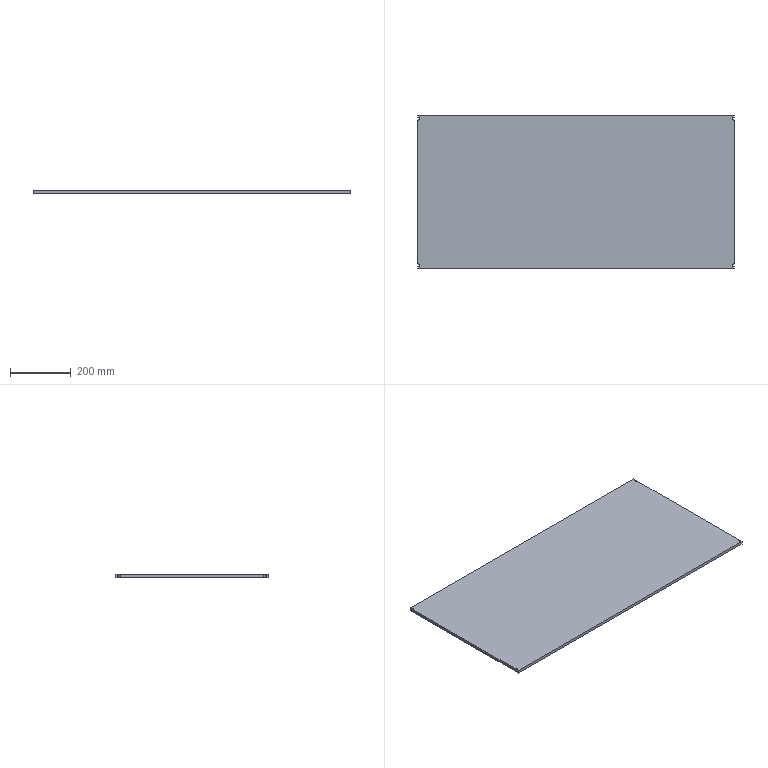Part | STEP file | 750038236 | 1 solid | 16 faces | box 1044 x 507 x 10 mm | volume 5291709 mm3 | plane 10 | cylinder 6 | commonest cylinder face diameters 10 x6
STEP:
#1=CARTESIAN_POINT('',(-517.5,-242.5,0.));
#2=VERTEX_POINT('',#1);
#3=CARTESIAN_POINT('',(-522.,-237.525,0.));
#4=VERTEX_POINT('',#3);
#5=CARTESIAN_POINT('',(-522.5,-242.5,0.));
#6=DIRECTION('',(0.,0.,1.));
#7=DIRECTION('',(1.,0.,0.));
#8=AXIS2_PLACEMENT_3D('',#5,#6,#7);
#9=CIRCLE('',#8,5.);
#10=EDGE_CURVE('',#2,#4,#9,.T.);
#11=ORIENTED_EDGE('',*,*,#10,.F.);
#12=CARTESIAN_POINT('',(-517.5,-242.5,10.));
#13=VERTEX_POINT('',#12);
#14=CARTESIAN_POINT('',(-517.5,-242.5,-54990.));
#15=DIRECTION('',(0.,0.,1.));
#16=VECTOR('',#15,1000.);
#17=LINE('',#14,#16);
#18=EDGE_CURVE('',#2,#13,#17,.T.);
#19=ORIENTED_EDGE('',*,*,#18,.T.);
#20=CARTESIAN_POINT('',(-522.,-237.525,10.));
#21=VERTEX_POINT('',#20);
#22=CARTESIAN_POINT('',(-522.5,-242.5,10.));
#23=DIRECTION('',(0.,0.,-1.));
#24=DIRECTION('',(1.,0.,0.));
#25=AXIS2_PLACEMENT_3D('',#22,#23,#24);
#26=CIRCLE('',#25,5.);
#27=EDGE_CURVE('',#21,#13,#26,.T.);
#28=ORIENTED_EDGE('',*,*,#27,.F.);
#29=CARTESIAN_POINT('',(-522.,-237.525,-54990.));
#30=DIRECTION('',(0.,0.,1.));
#31=VECTOR('',#30,1000.);
#32=LINE('',#29,#31);
#33=EDGE_CURVE('',#4,#21,#32,.T.);
#34=ORIENTED_EDGE('',*,*,#33,.F.);
#35=EDGE_LOOP('',(#11,#19,#28,#34));
#36=FACE_OUTER_BOUND('',#35,.T.);
#37=CARTESIAN_POINT('',(-522.5,-242.5,-54990.));
#38=DIRECTION('',(0.,0.,1.));
#39=DIRECTION('',(1.,0.,0.));
#40=AXIS2_PLACEMENT_3D('',#37,#38,#39);
#41=CYLINDRICAL_SURFACE('',#40,5.);
#42=ADVANCED_FACE('',(#36),#41,.F.);
#43=CARTESIAN_POINT('',(-517.5,242.5,0.));
#44=VERTEX_POINT('',#43);
#45=CARTESIAN_POINT('',(-522.,247.475,0.));
#46=VERTEX_POINT('',#45);
#47=CARTESIAN_POINT('',(-522.5,242.5,0.));
#48=DIRECTION('',(0.,0.,1.));
#49=DIRECTION('',(1.,0.,0.));
#50=AXIS2_PLACEMENT_3D('',#47,#48,#49);
#51=CIRCLE('',#50,5.);
#52=EDGE_CURVE('',#44,#46,#51,.T.);
#53=ORIENTED_EDGE('',*,*,#52,.F.);
#54=CARTESIAN_POINT('',(-517.5,242.5,10.));
#55=VERTEX_POINT('',#54);
#56=CARTESIAN_POINT('',(-517.5,242.5,-54990.));
#57=DIRECTION('',(0.,0.,1.));
#58=VECTOR('',#57,1000.);
#59=LINE('',#56,#58);
#60=EDGE_CURVE('',#44,#55,#59,.T.);
#61=ORIENTED_EDGE('',*,*,#60,.T.);
#62=CARTESIAN_POINT('',(-522.,247.475,10.));
#63=VERTEX_POINT('',#62);
#64=CARTESIAN_POINT('',(-522.5,242.5,10.));
#65=DIRECTION('',(0.,0.,-1.));
#66=DIRECTION('',(1.,0.,0.));
#67=AXIS2_PLACEMENT_3D('',#64,#65,#66);
#68=CIRCLE('',#67,5.);
#69=EDGE_CURVE('',#63,#55,#68,.T.);
#70=ORIENTED_EDGE('',*,*,#69,.F.);
#71=CARTESIAN_POINT('',(-522.,247.475,-54990.));
#72=DIRECTION('',(0.,0.,1.));
#73=VECTOR('',#72,1000.);
#74=LINE('',#71,#73);
#75=EDGE_CURVE('',#46,#63,#74,.T.);
#76=ORIENTED_EDGE('',*,*,#75,.F.);
#77=EDGE_LOOP('',(#53,#61,#70,#76));
#78=FACE_OUTER_BOUND('',#77,.T.);
#79=CARTESIAN_POINT('',(-522.5,242.5,-54990.));
#80=DIRECTION('',(0.,0.,1.));
#81=DIRECTION('',(1.,0.,0.));
#82=AXIS2_PLACEMENT_3D('',#79,#80,#81);
#83=CYLINDRICAL_SURFACE('',#82,5.);
#84=ADVANCED_FACE('',(#78),#83,.F.);
#85=CARTESIAN_POINT('',(-522.,-253.5,10.));
#86=VERTEX_POINT('',#85);
#87=CARTESIAN_POINT('',(522.,-253.5,10.));
#88=VERTEX_POINT('',#87);
#89=CARTESIAN_POINT('',(0.,-253.5,10.));
#90=DIRECTION('',(1.,0.,0.));
#91=VECTOR('',#90,1000.);
#92=LINE('',#89,#91);
#93=EDGE_CURVE('',#86,#88,#92,.T.);
#94=ORIENTED_EDGE('',*,*,#93,.T.);
#95=CARTESIAN_POINT('',(522.,-247.475,10.));
#96=VERTEX_POINT('',#95);
#97=CARTESIAN_POINT('',(522.,0.,10.));
#98=DIRECTION('',(0.,1.,0.));
#99=VECTOR('',#98,1000.);
#100=LINE('',#97,#99);
#101=EDGE_CURVE('',#88,#96,#100,.T.);
#102=ORIENTED_EDGE('',*,*,#101,.T.);
#103=CARTESIAN_POINT('',(522.,-237.525,10.));
#104=VERTEX_POINT('',#103);
#105=CARTESIAN_POINT('',(522.5,-242.5,10.));
#106=DIRECTION('',(0.,0.,-1.));
#107=DIRECTION('',(1.,0.,0.));
#108=AXIS2_PLACEMENT_3D('',#105,#106,#107);
#109=CIRCLE('',#108,5.);
#110=EDGE_CURVE('',#96,#104,#109,.T.);
#111=ORIENTED_EDGE('',*,*,#110,.T.);
#112=CARTESIAN_POINT('',(522.,237.525,10.));
#113=VERTEX_POINT('',#112);
#114=CARTESIAN_POINT('',(522.,0.,10.));
#115=DIRECTION('',(0.,1.,0.));
#116=VECTOR('',#115,1000.);
#117=LINE('',#114,#116);
#118=EDGE_CURVE('',#104,#113,#117,.T.);
#119=ORIENTED_EDGE('',*,*,#118,.T.);
#120=CARTESIAN_POINT('',(522.,247.475,10.));
#121=VERTEX_POINT('',#120);
#122=CARTESIAN_POINT('',(522.5,242.5,10.));
#123=DIRECTION('',(0.,0.,-1.));
#124=DIRECTION('',(1.,0.,0.));
#125=AXIS2_PLACEMENT_3D('',#122,#123,#124);
#126=CIRCLE('',#125,5.);
#127=EDGE_CURVE('',#113,#121,#126,.T.);
#128=ORIENTED_EDGE('',*,*,#127,.T.);
#129=CARTESIAN_POINT('',(522.,253.5,10.));
#130=VERTEX_POINT('',#129);
#131=CARTESIAN_POINT('',(522.,0.,10.));
#132=DIRECTION('',(0.,1.,0.));
#133=VECTOR('',#132,1000.);
#134=LINE('',#131,#133);
#135=EDGE_CURVE('',#121,#130,#134,.T.);
#136=ORIENTED_EDGE('',*,*,#135,.T.);
#137=CARTESIAN_POINT('',(-522.,253.5,10.));
#138=VERTEX_POINT('',#137);
#139=CARTESIAN_POINT('',(0.,253.5,10.));
#140=DIRECTION('',(-1.,0.,0.));
#141=VECTOR('',#140,1000.);
#142=LINE('',#139,#141);
#143=EDGE_CURVE('',#130,#138,#142,.T.);
#144=ORIENTED_EDGE('',*,*,#143,.T.);
#145=CARTESIAN_POINT('',(-522.,0.,10.));
#146=DIRECTION('',(0.,-1.,0.));
#147=VECTOR('',#146,1000.);
#148=LINE('',#145,#147);
#149=EDGE_CURVE('',#138,#63,#148,.T.);
#150=ORIENTED_EDGE('',*,*,#149,.T.);
#151=ORIENTED_EDGE('',*,*,#69,.T.);
#152=CARTESIAN_POINT('',(-522.,237.525,10.));
#153=VERTEX_POINT('',#152);
#154=CARTESIAN_POINT('',(-522.5,242.5,10.));
#155=DIRECTION('',(0.,0.,-1.));
#156=DIRECTION('',(1.,0.,0.));
#157=AXIS2_PLACEMENT_3D('',#154,#155,#156);
#158=CIRCLE('',#157,5.);
#159=EDGE_CURVE('',#55,#153,#158,.T.);
#160=ORIENTED_EDGE('',*,*,#159,.T.);
#161=CARTESIAN_POINT('',(-522.,0.,10.));
#162=DIRECTION('',(0.,-1.,0.));
#163=VECTOR('',#162,1000.);
#164=LINE('',#161,#163);
#165=EDGE_CURVE('',#153,#21,#164,.T.);
#166=ORIENTED_EDGE('',*,*,#165,.T.);
#167=ORIENTED_EDGE('',*,*,#27,.T.);
#168=CARTESIAN_POINT('',(-522.,-247.475,10.));
#169=VERTEX_POINT('',#168);
#170=CARTESIAN_POINT('',(-522.5,-242.5,10.));
#171=DIRECTION('',(0.,0.,-1.));
#172=DIRECTION('',(1.,0.,0.));
#173=AXIS2_PLACEMENT_3D('',#170,#171,#172);
#174=CIRCLE('',#173,5.);
#175=EDGE_CURVE('',#13,#169,#174,.T.);
#176=ORIENTED_EDGE('',*,*,#175,.T.);
#177=CARTESIAN_POINT('',(-522.,0.,10.));
#178=DIRECTION('',(0.,-1.,0.));
#179=VECTOR('',#178,1000.);
#180=LINE('',#177,#179);
#181=EDGE_CURVE('',#169,#86,#180,.T.);
#182=ORIENTED_EDGE('',*,*,#181,.T.);
#183=EDGE_LOOP('',(#94,#102,#111,#119,#128,#136,#144,#150,#151,#160,#166,#167,#176,#182));
#184=FACE_OUTER_BOUND('',#183,.T.);
#185=CARTESIAN_POINT('',(0.,0.,10.));
#186=DIRECTION('',(0.,0.,1.));
#187=DIRECTION('',(1.,0.,0.));
#188=AXIS2_PLACEMENT_3D('',#185,#186,#187);
#189=PLANE('',#188);
#190=ADVANCED_FACE('',(#184),#189,.T.);
#191=CARTESIAN_POINT('',(522.,-247.475,0.));
#192=VERTEX_POINT('',#191);
#193=CARTESIAN_POINT('',(522.,-247.475,10.));
#194=DIRECTION('',(0.,0.,-1.));
#195=VECTOR('',#194,1000.);
#196=LINE('',#193,#195);
#197=EDGE_CURVE('',#96,#192,#196,.T.);
#198=ORIENTED_EDGE('',*,*,#197,.F.);
#199=ORIENTED_EDGE('',*,*,#101,.F.);
#200=CARTESIAN_POINT('',(522.,-253.5,0.));
#201=VERTEX_POINT('',#200);
#202=CARTESIAN_POINT('',(522.,-253.5,10.));
#203=DIRECTION('',(0.,0.,1.));
#204=VECTOR('',#203,1000.);
#205=LINE('',#202,#204);
#206=EDGE_CURVE('',#201,#88,#205,.T.);
#207=ORIENTED_EDGE('',*,*,#206,.F.);
#208=CARTESIAN_POINT('',(522.,-253.5,0.));
#209=DIRECTION('',(0.,-1.,0.));
#210=VECTOR('',#209,1000.);
#211=LINE('',#208,#210);
#212=EDGE_CURVE('',#192,#201,#211,.T.);
#213=ORIENTED_EDGE('',*,*,#212,.F.);
#214=EDGE_LOOP('',(#198,#199,#207,#213));
#215=FACE_OUTER_BOUND('',#214,.T.);
#216=CARTESIAN_POINT('',(522.,-253.5,10.));
#217=DIRECTION('',(-1.,0.,0.));
#218=DIRECTION('',(0.,0.,1.));
#219=AXIS2_PLACEMENT_3D('',#216,#217,#218);
#220=PLANE('',#219);
#221=ADVANCED_FACE('',(#215),#220,.F.);
#222=ORIENTED_EDGE('',*,*,#206,.T.);
#223=ORIENTED_EDGE('',*,*,#93,.F.);
#224=CARTESIAN_POINT('',(-522.,-253.5,0.));
#225=VERTEX_POINT('',#224);
#226=CARTESIAN_POINT('',(-522.,-253.5,10.));
#227=DIRECTION('',(0.,0.,1.));
#228=VECTOR('',#227,1000.);
#229=LINE('',#226,#228);
#230=EDGE_CURVE('',#225,#86,#229,.T.);
#231=ORIENTED_EDGE('',*,*,#230,.F.);
#232=CARTESIAN_POINT('',(-522.,-253.5,0.));
#233=DIRECTION('',(-1.,0.,0.));
#234=VECTOR('',#233,1000.);
#235=LINE('',#232,#234);
#236=EDGE_CURVE('',#201,#225,#235,.T.);
#237=ORIENTED_EDGE('',*,*,#236,.F.);
#238=EDGE_LOOP('',(#222,#223,#231,#237));
#239=FACE_OUTER_BOUND('',#238,.T.);
#240=CARTESIAN_POINT('',(-522.,-253.5,10.));
#241=DIRECTION('',(0.,1.,0.));
#242=DIRECTION('',(0.,0.,1.));
#243=AXIS2_PLACEMENT_3D('',#240,#241,#242);
#244=PLANE('',#243);
#245=ADVANCED_FACE('',(#239),#244,.F.);
#246=CARTESIAN_POINT('',(-522.,-247.475,0.));
#247=VERTEX_POINT('',#246);
#248=CARTESIAN_POINT('',(-522.,-247.475,10.));
#249=DIRECTION('',(0.,0.,1.));
#250=VECTOR('',#249,1000.);
#251=LINE('',#248,#250);
#252=EDGE_CURVE('',#247,#169,#251,.T.);
#253=ORIENTED_EDGE('',*,*,#252,.F.);
#254=CARTESIAN_POINT('',(-522.,253.5,0.));
#255=DIRECTION('',(0.,1.,0.));
#256=VECTOR('',#255,1000.);
#257=LINE('',#254,#256);
#258=EDGE_CURVE('',#225,#247,#257,.T.);
#259=ORIENTED_EDGE('',*,*,#258,.F.);
#260=ORIENTED_EDGE('',*,*,#230,.T.);
#261=ORIENTED_EDGE('',*,*,#181,.F.);
#262=EDGE_LOOP('',(#253,#259,#260,#261));
#263=FACE_OUTER_BOUND('',#262,.T.);
#264=CARTESIAN_POINT('',(-522.,253.5,10.));
#265=DIRECTION('',(1.,0.,0.));
#266=DIRECTION('',(0.,0.,-1.));
#267=AXIS2_PLACEMENT_3D('',#264,#265,#266);
#268=PLANE('',#267);
#269=ADVANCED_FACE('',(#263),#268,.F.);
#270=ORIENTED_EDGE('',*,*,#18,.F.);
#271=CARTESIAN_POINT('',(-522.5,-242.5,0.));
#272=DIRECTION('',(0.,0.,1.));
#273=DIRECTION('',(1.,0.,0.));
#274=AXIS2_PLACEMENT_3D('',#271,#272,#273);
#275=CIRCLE('',#274,5.);
#276=EDGE_CURVE('',#247,#2,#275,.T.);
#277=ORIENTED_EDGE('',*,*,#276,.F.);
#278=ORIENTED_EDGE('',*,*,#252,.T.);
#279=ORIENTED_EDGE('',*,*,#175,.F.);
#280=EDGE_LOOP('',(#270,#277,#278,#279));
#281=FACE_OUTER_BOUND('',#280,.T.);
#282=CARTESIAN_POINT('',(-522.5,-242.5,-54990.));
#283=DIRECTION('',(0.,0.,1.));
#284=DIRECTION('',(1.,0.,0.));
#285=AXIS2_PLACEMENT_3D('',#282,#283,#284);
#286=CYLINDRICAL_SURFACE('',#285,5.);
#287=ADVANCED_FACE('',(#281),#286,.F.);
#288=CARTESIAN_POINT('',(-522.,237.525,0.));
#289=VERTEX_POINT('',#288);
#290=CARTESIAN_POINT('',(-522.,237.525,10.));
#291=DIRECTION('',(0.,0.,1.));
#292=VECTOR('',#291,1000.);
#293=LINE('',#290,#292);
#294=EDGE_CURVE('',#289,#153,#293,.T.);
#295=ORIENTED_EDGE('',*,*,#294,.F.);
#296=CARTESIAN_POINT('',(-522.,253.5,0.));
#297=DIRECTION('',(0.,1.,0.));
#298=VECTOR('',#297,1000.);
#299=LINE('',#296,#298);
#300=EDGE_CURVE('',#4,#289,#299,.T.);
#301=ORIENTED_EDGE('',*,*,#300,.F.);
#302=ORIENTED_EDGE('',*,*,#33,.T.);
#303=ORIENTED_EDGE('',*,*,#165,.F.);
#304=EDGE_LOOP('',(#295,#301,#302,#303));
#305=FACE_OUTER_BOUND('',#304,.T.);
#306=CARTESIAN_POINT('',(-522.,253.5,10.));
#307=DIRECTION('',(1.,0.,0.));
#308=DIRECTION('',(0.,0.,-1.));
#309=AXIS2_PLACEMENT_3D('',#306,#307,#308);
#310=PLANE('',#309);
#311=ADVANCED_FACE('',(#305),#310,.F.);
#312=ORIENTED_EDGE('',*,*,#60,.F.);
#313=CARTESIAN_POINT('',(-522.5,242.5,0.));
#314=DIRECTION('',(0.,0.,1.));
#315=DIRECTION('',(1.,0.,0.));
#316=AXIS2_PLACEMENT_3D('',#313,#314,#315);
#317=CIRCLE('',#316,5.);
#318=EDGE_CURVE('',#289,#44,#317,.T.);
#319=ORIENTED_EDGE('',*,*,#318,.F.);
#320=ORIENTED_EDGE('',*,*,#294,.T.);
#321=ORIENTED_EDGE('',*,*,#159,.F.);
#322=EDGE_LOOP('',(#312,#319,#320,#321));
#323=FACE_OUTER_BOUND('',#322,.T.);
#324=CARTESIAN_POINT('',(-522.5,242.5,-54990.));
#325=DIRECTION('',(0.,0.,1.));
#326=DIRECTION('',(1.,0.,0.));
#327=AXIS2_PLACEMENT_3D('',#324,#325,#326);
#328=CYLINDRICAL_SURFACE('',#327,5.);
#329=ADVANCED_FACE('',(#323),#328,.F.);
#330=ORIENTED_EDGE('',*,*,#75,.T.);
#331=ORIENTED_EDGE('',*,*,#149,.F.);
#332=CARTESIAN_POINT('',(-522.,253.5,0.));
#333=VERTEX_POINT('',#332);
#334=CARTESIAN_POINT('',(-522.,253.5,10.));
#335=DIRECTION('',(0.,0.,1.));
#336=VECTOR('',#335,1000.);
#337=LINE('',#334,#336);
#338=EDGE_CURVE('',#333,#138,#337,.T.);
#339=ORIENTED_EDGE('',*,*,#338,.F.);
#340=CARTESIAN_POINT('',(-522.,253.5,0.));
#341=DIRECTION('',(0.,1.,0.));
#342=VECTOR('',#341,1000.);
#343=LINE('',#340,#342);
#344=EDGE_CURVE('',#46,#333,#343,.T.);
#345=ORIENTED_EDGE('',*,*,#344,.F.);
#346=EDGE_LOOP('',(#330,#331,#339,#345));
#347=FACE_OUTER_BOUND('',#346,.T.);
#348=CARTESIAN_POINT('',(-522.,253.5,10.));
#349=DIRECTION('',(1.,0.,0.));
#350=DIRECTION('',(0.,0.,-1.));
#351=AXIS2_PLACEMENT_3D('',#348,#349,#350);
#352=PLANE('',#351);
#353=ADVANCED_FACE('',(#347),#352,.F.);
#354=ORIENTED_EDGE('',*,*,#338,.T.);
#355=ORIENTED_EDGE('',*,*,#143,.F.);
#356=CARTESIAN_POINT('',(522.,253.5,0.));
#357=VERTEX_POINT('',#356);
#358=CARTESIAN_POINT('',(522.,253.5,10.));
#359=DIRECTION('',(0.,0.,1.));
#360=VECTOR('',#359,1000.);
#361=LINE('',#358,#360);
#362=EDGE_CURVE('',#357,#130,#361,.T.);
#363=ORIENTED_EDGE('',*,*,#362,.F.);
#364=CARTESIAN_POINT('',(522.,253.5,0.));
#365=DIRECTION('',(1.,0.,0.));
#366=VECTOR('',#365,1000.);
#367=LINE('',#364,#366);
#368=EDGE_CURVE('',#333,#357,#367,.T.);
#369=ORIENTED_EDGE('',*,*,#368,.F.);
#370=EDGE_LOOP('',(#354,#355,#363,#369));
#371=FACE_OUTER_BOUND('',#370,.T.);
#372=CARTESIAN_POINT('',(522.,253.5,10.));
#373=DIRECTION('',(0.,-1.,0.));
#374=DIRECTION('',(0.,0.,-1.));
#375=AXIS2_PLACEMENT_3D('',#372,#373,#374);
#376=PLANE('',#375);
#377=ADVANCED_FACE('',(#371),#376,.F.);
#378=CARTESIAN_POINT('',(522.,247.475,0.));
#379=VERTEX_POINT('',#378);
#380=CARTESIAN_POINT('',(522.,247.475,10.));
#381=DIRECTION('',(0.,0.,1.));
#382=VECTOR('',#381,1000.);
#383=LINE('',#380,#382);
#384=EDGE_CURVE('',#379,#121,#383,.T.);
#385=ORIENTED_EDGE('',*,*,#384,.F.);
#386=CARTESIAN_POINT('',(522.,-253.5,0.));
#387=DIRECTION('',(0.,-1.,0.));
#388=VECTOR('',#387,1000.);
#389=LINE('',#386,#388);
#390=EDGE_CURVE('',#357,#379,#389,.T.);
#391=ORIENTED_EDGE('',*,*,#390,.F.);
#392=ORIENTED_EDGE('',*,*,#362,.T.);
#393=ORIENTED_EDGE('',*,*,#135,.F.);
#394=EDGE_LOOP('',(#385,#391,#392,#393));
#395=FACE_OUTER_BOUND('',#394,.T.);
#396=CARTESIAN_POINT('',(522.,-253.5,10.));
#397=DIRECTION('',(-1.,0.,0.));
#398=DIRECTION('',(0.,0.,1.));
#399=AXIS2_PLACEMENT_3D('',#396,#397,#398);
#400=PLANE('',#399);
#401=ADVANCED_FACE('',(#395),#400,.F.);
#402=ORIENTED_EDGE('',*,*,#384,.T.);
#403=ORIENTED_EDGE('',*,*,#127,.F.);
#404=CARTESIAN_POINT('',(522.,237.525,0.));
#405=VERTEX_POINT('',#404);
#406=CARTESIAN_POINT('',(522.,237.525,-54990.));
#407=DIRECTION('',(0.,0.,1.));
#408=VECTOR('',#407,1000.);
#409=LINE('',#406,#408);
#410=EDGE_CURVE('',#405,#113,#409,.T.);
#411=ORIENTED_EDGE('',*,*,#410,.F.);
#412=CARTESIAN_POINT('',(522.5,242.5,0.));
#413=DIRECTION('',(0.,0.,1.));
#414=DIRECTION('',(1.,0.,0.));
#415=AXIS2_PLACEMENT_3D('',#412,#413,#414);
#416=CIRCLE('',#415,5.);
#417=EDGE_CURVE('',#379,#405,#416,.T.);
#418=ORIENTED_EDGE('',*,*,#417,.F.);
#419=EDGE_LOOP('',(#402,#403,#411,#418));
#420=FACE_OUTER_BOUND('',#419,.T.);
#421=CARTESIAN_POINT('',(522.5,242.5,-54990.));
#422=DIRECTION('',(0.,0.,1.));
#423=DIRECTION('',(1.,0.,0.));
#424=AXIS2_PLACEMENT_3D('',#421,#422,#423);
#425=CYLINDRICAL_SURFACE('',#424,5.);
#426=ADVANCED_FACE('',(#420),#425,.F.);
#427=CARTESIAN_POINT('',(522.,-237.525,0.));
#428=VERTEX_POINT('',#427);
#429=CARTESIAN_POINT('',(522.,-237.525,10.));
#430=DIRECTION('',(0.,0.,1.));
#431=VECTOR('',#430,1000.);
#432=LINE('',#429,#431);
#433=EDGE_CURVE('',#428,#104,#432,.T.);
#434=ORIENTED_EDGE('',*,*,#433,.F.);
#435=CARTESIAN_POINT('',(522.,-253.5,0.));
#436=DIRECTION('',(0.,-1.,0.));
#437=VECTOR('',#436,1000.);
#438=LINE('',#435,#437);
#439=EDGE_CURVE('',#405,#428,#438,.T.);
#440=ORIENTED_EDGE('',*,*,#439,.F.);
#441=ORIENTED_EDGE('',*,*,#410,.T.);
#442=ORIENTED_EDGE('',*,*,#118,.F.);
#443=EDGE_LOOP('',(#434,#440,#441,#442));
#444=FACE_OUTER_BOUND('',#443,.T.);
#445=CARTESIAN_POINT('',(522.,-253.5,10.));
#446=DIRECTION('',(-1.,0.,0.));
#447=DIRECTION('',(0.,0.,1.));
#448=AXIS2_PLACEMENT_3D('',#445,#446,#447);
#449=PLANE('',#448);
#450=ADVANCED_FACE('',(#444),#449,.F.);
#451=ORIENTED_EDGE('',*,*,#433,.T.);
#452=ORIENTED_EDGE('',*,*,#110,.F.);
#453=ORIENTED_EDGE('',*,*,#197,.T.);
#454=CARTESIAN_POINT('',(522.5,-242.5,0.));
#455=DIRECTION('',(0.,0.,1.));
#456=DIRECTION('',(1.,0.,0.));
#457=AXIS2_PLACEMENT_3D('',#454,#455,#456);
#458=CIRCLE('',#457,5.);
#459=EDGE_CURVE('',#428,#192,#458,.T.);
#460=ORIENTED_EDGE('',*,*,#459,.F.);
#461=EDGE_LOOP('',(#451,#452,#453,#460));
#462=FACE_OUTER_BOUND('',#461,.T.);
#463=CARTESIAN_POINT('',(522.5,-242.5,-54990.));
#464=DIRECTION('',(0.,0.,1.));
#465=DIRECTION('',(1.,0.,0.));
#466=AXIS2_PLACEMENT_3D('',#463,#464,#465);
#467=CYLINDRICAL_SURFACE('',#466,5.);
#468=ADVANCED_FACE('',(#462),#467,.F.);
#469=ORIENTED_EDGE('',*,*,#459,.T.);
#470=ORIENTED_EDGE('',*,*,#212,.T.);
#471=ORIENTED_EDGE('',*,*,#236,.T.);
#472=ORIENTED_EDGE('',*,*,#258,.T.);
#473=ORIENTED_EDGE('',*,*,#276,.T.);
#474=ORIENTED_EDGE('',*,*,#10,.T.);
#475=ORIENTED_EDGE('',*,*,#300,.T.);
#476=ORIENTED_EDGE('',*,*,#318,.T.);
#477=ORIENTED_EDGE('',*,*,#52,.T.);
#478=ORIENTED_EDGE('',*,*,#344,.T.);
#479=ORIENTED_EDGE('',*,*,#368,.T.);
#480=ORIENTED_EDGE('',*,*,#390,.T.);
#481=ORIENTED_EDGE('',*,*,#417,.T.);
#482=ORIENTED_EDGE('',*,*,#439,.T.);
#483=EDGE_LOOP('',(#469,#470,#471,#472,#473,#474,#475,#476,#477,#478,#479,#480,#481,#482));
#484=FACE_OUTER_BOUND('',#483,.T.);
#485=CARTESIAN_POINT('',(0.,0.,0.));
#486=DIRECTION('',(0.,0.,1.));
#487=DIRECTION('',(1.,0.,0.));
#488=AXIS2_PLACEMENT_3D('',#485,#486,#487);
#489=PLANE('',#488);
#490=ADVANCED_FACE('',(#484),#489,.F.);
#491=CLOSED_SHELL('',(#42,#84,#190,#221,#245,#269,#287,#311,#329,#353,#377,#401,#426,#450,#468,#490));
#492=MANIFOLD_SOLID_BREP('',#491);
#493=CARTESIAN_POINT('',(0.,0.,0.));
#494=DIRECTION('',(0.,0.,1.));
#495=DIRECTION('',(1.,0.,0.));
#496=AXIS2_PLACEMENT_3D('',#493,#494,#495);
#497=(LENGTH_UNIT()NAMED_UNIT(*)SI_UNIT(.MILLI.,.METRE.));
#498=UNCERTAINTY_MEASURE_WITH_UNIT(LENGTH_MEASURE(0.00001),#497,'','');
#499=(NAMED_UNIT(*)PLANE_ANGLE_UNIT()SI_UNIT($,.RADIAN.));
#500=(NAMED_UNIT(*)SI_UNIT($,.STERADIAN.)SOLID_ANGLE_UNIT());
#501=(GEOMETRIC_REPRESENTATION_CONTEXT(3)GLOBAL_UNCERTAINTY_ASSIGNED_CONTEXT((#498))GLOBAL_UNIT_ASSIGNED_CONTEXT((#497,#499,#500))REPRESENTATION_CONTEXT('',''));
#502=ADVANCED_BREP_SHAPE_REPRESENTATION('',(#492,#496),#501);